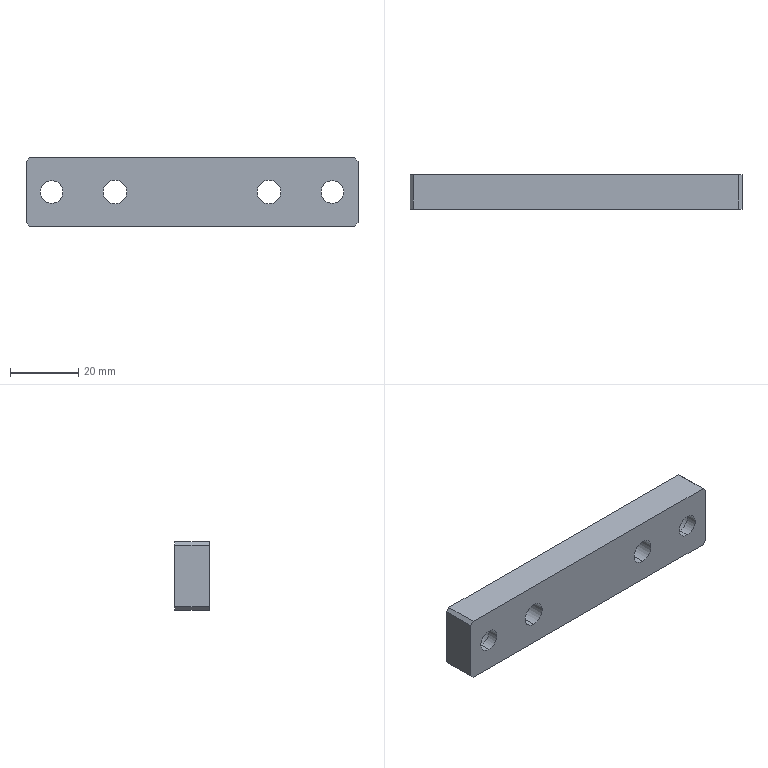Part | SolidWorks | features HoleWzd 2, Chamfer 1, Extrusion 1, ICE 1 | 1 solid | 24 faces | box 97 x 10 x 20 mm | volume 17099 mm3 | cylinder 12 | plane 12 | commonest cylinder face diameters 6.6 x4 7 x4 11 x4
STEP:
#1=CARTESIAN_POINT('',(-41.,-1.8,-5.5));
#2=VERTEX_POINT('',#1);
#3=CARTESIAN_POINT('',(-41.,-1.8,5.5));
#4=VERTEX_POINT('',#3);
#5=CARTESIAN_POINT('',(-41.,-1.8,0.));
#6=DIRECTION('',(0.,1.,0.));
#7=DIRECTION('',(0.,0.,1.));
#8=AXIS2_PLACEMENT_3D('',#5,#6,#7);
#9=CIRCLE('',#8,5.5);
#10=EDGE_CURVE('',#2,#4,#9,.T.);
#11=ORIENTED_EDGE('',*,*,#10,.F.);
#12=CARTESIAN_POINT('',(-41.,5.,-5.5));
#13=VERTEX_POINT('',#12);
#14=CARTESIAN_POINT('',(-41.,5.,-5.5));
#15=DIRECTION('',(0.,1.,0.));
#16=VECTOR('',#15,1000.);
#17=LINE('',#14,#16);
#18=EDGE_CURVE('',#2,#13,#17,.T.);
#19=ORIENTED_EDGE('',*,*,#18,.T.);
#20=CARTESIAN_POINT('',(-41.,5.,5.5));
#21=VERTEX_POINT('',#20);
#22=CARTESIAN_POINT('',(-41.,5.,0.));
#23=DIRECTION('',(0.,1.,0.));
#24=DIRECTION('',(0.,0.,1.));
#25=AXIS2_PLACEMENT_3D('',#22,#23,#24);
#26=CIRCLE('',#25,5.5);
#27=EDGE_CURVE('',#13,#21,#26,.T.);
#28=ORIENTED_EDGE('',*,*,#27,.T.);
#29=CARTESIAN_POINT('',(-41.,5.,5.5));
#30=DIRECTION('',(0.,1.,0.));
#31=VECTOR('',#30,1000.);
#32=LINE('',#29,#31);
#33=EDGE_CURVE('',#4,#21,#32,.T.);
#34=ORIENTED_EDGE('',*,*,#33,.F.);
#35=EDGE_LOOP('',(#11,#19,#28,#34));
#36=FACE_OUTER_BOUND('',#35,.T.);
#37=CARTESIAN_POINT('',(-41.,5.,0.));
#38=DIRECTION('',(0.,1.,0.));
#39=DIRECTION('',(0.,0.,1.));
#40=AXIS2_PLACEMENT_3D('',#37,#38,#39);
#41=CYLINDRICAL_SURFACE('',#40,5.5);
#42=ADVANCED_FACE('',(#36),#41,.F.);
#43=CARTESIAN_POINT('',(-41.,-5.,-3.3));
#44=VERTEX_POINT('',#43);
#45=CARTESIAN_POINT('',(-41.,-5.,3.3));
#46=VERTEX_POINT('',#45);
#47=CARTESIAN_POINT('',(-41.,-5.,0.));
#48=DIRECTION('',(0.,1.,0.));
#49=DIRECTION('',(0.,0.,1.));
#50=AXIS2_PLACEMENT_3D('',#47,#48,#49);
#51=CIRCLE('',#50,3.3);
#52=EDGE_CURVE('',#44,#46,#51,.T.);
#53=ORIENTED_EDGE('',*,*,#52,.F.);
#54=CARTESIAN_POINT('',(-41.,-1.8,-3.3));
#55=VERTEX_POINT('',#54);
#56=CARTESIAN_POINT('',(-41.,5.,-3.3));
#57=DIRECTION('',(0.,1.,0.));
#58=VECTOR('',#57,1000.);
#59=LINE('',#56,#58);
#60=EDGE_CURVE('',#44,#55,#59,.T.);
#61=ORIENTED_EDGE('',*,*,#60,.T.);
#62=CARTESIAN_POINT('',(-41.,-1.8,3.3));
#63=VERTEX_POINT('',#62);
#64=CARTESIAN_POINT('',(-41.,-1.8,0.));
#65=DIRECTION('',(0.,1.,0.));
#66=DIRECTION('',(0.,0.,1.));
#67=AXIS2_PLACEMENT_3D('',#64,#65,#66);
#68=CIRCLE('',#67,3.3);
#69=EDGE_CURVE('',#55,#63,#68,.T.);
#70=ORIENTED_EDGE('',*,*,#69,.T.);
#71=CARTESIAN_POINT('',(-41.,5.,3.3));
#72=DIRECTION('',(0.,1.,0.));
#73=VECTOR('',#72,1000.);
#74=LINE('',#71,#73);
#75=EDGE_CURVE('',#46,#63,#74,.T.);
#76=ORIENTED_EDGE('',*,*,#75,.F.);
#77=EDGE_LOOP('',(#53,#61,#70,#76));
#78=FACE_OUTER_BOUND('',#77,.T.);
#79=CARTESIAN_POINT('',(-41.,5.,0.));
#80=DIRECTION('',(0.,1.,0.));
#81=DIRECTION('',(0.,0.,1.));
#82=AXIS2_PLACEMENT_3D('',#79,#80,#81);
#83=CYLINDRICAL_SURFACE('',#82,3.3);
#84=ADVANCED_FACE('',(#78),#83,.F.);
#85=CARTESIAN_POINT('',(41.,-1.8,-5.5));
#86=VERTEX_POINT('',#85);
#87=CARTESIAN_POINT('',(41.,-1.8,5.5));
#88=VERTEX_POINT('',#87);
#89=CARTESIAN_POINT('',(41.,-1.8,0.));
#90=DIRECTION('',(0.,1.,0.));
#91=DIRECTION('',(0.,0.,1.));
#92=AXIS2_PLACEMENT_3D('',#89,#90,#91);
#93=CIRCLE('',#92,5.5);
#94=EDGE_CURVE('',#86,#88,#93,.T.);
#95=ORIENTED_EDGE('',*,*,#94,.F.);
#96=CARTESIAN_POINT('',(41.,5.,-5.5));
#97=VERTEX_POINT('',#96);
#98=CARTESIAN_POINT('',(41.,5.,-5.5));
#99=DIRECTION('',(0.,1.,0.));
#100=VECTOR('',#99,1000.);
#101=LINE('',#98,#100);
#102=EDGE_CURVE('',#86,#97,#101,.T.);
#103=ORIENTED_EDGE('',*,*,#102,.T.);
#104=CARTESIAN_POINT('',(41.,5.,5.5));
#105=VERTEX_POINT('',#104);
#106=CARTESIAN_POINT('',(41.,5.,0.));
#107=DIRECTION('',(0.,1.,0.));
#108=DIRECTION('',(0.,0.,1.));
#109=AXIS2_PLACEMENT_3D('',#106,#107,#108);
#110=CIRCLE('',#109,5.5);
#111=EDGE_CURVE('',#97,#105,#110,.T.);
#112=ORIENTED_EDGE('',*,*,#111,.T.);
#113=CARTESIAN_POINT('',(41.,5.,5.5));
#114=DIRECTION('',(0.,1.,0.));
#115=VECTOR('',#114,1000.);
#116=LINE('',#113,#115);
#117=EDGE_CURVE('',#88,#105,#116,.T.);
#118=ORIENTED_EDGE('',*,*,#117,.F.);
#119=EDGE_LOOP('',(#95,#103,#112,#118));
#120=FACE_OUTER_BOUND('',#119,.T.);
#121=CARTESIAN_POINT('',(41.,5.,0.));
#122=DIRECTION('',(0.,1.,0.));
#123=DIRECTION('',(0.,0.,1.));
#124=AXIS2_PLACEMENT_3D('',#121,#122,#123);
#125=CYLINDRICAL_SURFACE('',#124,5.5);
#126=ADVANCED_FACE('',(#120),#125,.F.);
#127=CARTESIAN_POINT('',(41.,-5.,-3.3));
#128=VERTEX_POINT('',#127);
#129=CARTESIAN_POINT('',(41.,-5.,3.3));
#130=VERTEX_POINT('',#129);
#131=CARTESIAN_POINT('',(41.,-5.,0.));
#132=DIRECTION('',(0.,1.,0.));
#133=DIRECTION('',(0.,0.,1.));
#134=AXIS2_PLACEMENT_3D('',#131,#132,#133);
#135=CIRCLE('',#134,3.3);
#136=EDGE_CURVE('',#128,#130,#135,.T.);
#137=ORIENTED_EDGE('',*,*,#136,.F.);
#138=CARTESIAN_POINT('',(41.,-1.8,-3.3));
#139=VERTEX_POINT('',#138);
#140=CARTESIAN_POINT('',(41.,5.,-3.3));
#141=DIRECTION('',(0.,1.,0.));
#142=VECTOR('',#141,1000.);
#143=LINE('',#140,#142);
#144=EDGE_CURVE('',#128,#139,#143,.T.);
#145=ORIENTED_EDGE('',*,*,#144,.T.);
#146=CARTESIAN_POINT('',(41.,-1.8,3.3));
#147=VERTEX_POINT('',#146);
#148=CARTESIAN_POINT('',(41.,-1.8,0.));
#149=DIRECTION('',(0.,1.,0.));
#150=DIRECTION('',(0.,0.,1.));
#151=AXIS2_PLACEMENT_3D('',#148,#149,#150);
#152=CIRCLE('',#151,3.3);
#153=EDGE_CURVE('',#139,#147,#152,.T.);
#154=ORIENTED_EDGE('',*,*,#153,.T.);
#155=CARTESIAN_POINT('',(41.,5.,3.3));
#156=DIRECTION('',(0.,1.,0.));
#157=VECTOR('',#156,1000.);
#158=LINE('',#155,#157);
#159=EDGE_CURVE('',#130,#147,#158,.T.);
#160=ORIENTED_EDGE('',*,*,#159,.F.);
#161=EDGE_LOOP('',(#137,#145,#154,#160));
#162=FACE_OUTER_BOUND('',#161,.T.);
#163=CARTESIAN_POINT('',(41.,5.,0.));
#164=DIRECTION('',(0.,1.,0.));
#165=DIRECTION('',(0.,0.,1.));
#166=AXIS2_PLACEMENT_3D('',#163,#164,#165);
#167=CYLINDRICAL_SURFACE('',#166,3.3);
#168=ADVANCED_FACE('',(#162),#167,.F.);
#169=CARTESIAN_POINT('',(-22.5,-5.,-3.5));
#170=VERTEX_POINT('',#169);
#171=CARTESIAN_POINT('',(-22.5,-5.,3.5));
#172=VERTEX_POINT('',#171);
#173=CARTESIAN_POINT('',(-22.5,-5.,0.));
#174=DIRECTION('',(0.,1.,0.));
#175=DIRECTION('',(0.,0.,1.));
#176=AXIS2_PLACEMENT_3D('',#173,#174,#175);
#177=CIRCLE('',#176,3.5);
#178=EDGE_CURVE('',#170,#172,#177,.T.);
#179=ORIENTED_EDGE('',*,*,#178,.F.);
#180=CARTESIAN_POINT('',(-22.5,5.,-3.5));
#181=VERTEX_POINT('',#180);
#182=CARTESIAN_POINT('',(-22.5,5.,-3.5));
#183=DIRECTION('',(0.,1.,0.));
#184=VECTOR('',#183,1000.);
#185=LINE('',#182,#184);
#186=EDGE_CURVE('',#170,#181,#185,.T.);
#187=ORIENTED_EDGE('',*,*,#186,.T.);
#188=CARTESIAN_POINT('',(-22.5,5.,3.5));
#189=VERTEX_POINT('',#188);
#190=CARTESIAN_POINT('',(-22.5,5.,0.));
#191=DIRECTION('',(0.,1.,0.));
#192=DIRECTION('',(0.,0.,1.));
#193=AXIS2_PLACEMENT_3D('',#190,#191,#192);
#194=CIRCLE('',#193,3.5);
#195=EDGE_CURVE('',#181,#189,#194,.T.);
#196=ORIENTED_EDGE('',*,*,#195,.T.);
#197=CARTESIAN_POINT('',(-22.5,5.,3.5));
#198=DIRECTION('',(0.,1.,0.));
#199=VECTOR('',#198,1000.);
#200=LINE('',#197,#199);
#201=EDGE_CURVE('',#172,#189,#200,.T.);
#202=ORIENTED_EDGE('',*,*,#201,.F.);
#203=EDGE_LOOP('',(#179,#187,#196,#202));
#204=FACE_OUTER_BOUND('',#203,.T.);
#205=CARTESIAN_POINT('',(-22.5,5.,0.));
#206=DIRECTION('',(0.,1.,0.));
#207=DIRECTION('',(0.,0.,1.));
#208=AXIS2_PLACEMENT_3D('',#205,#206,#207);
#209=CYLINDRICAL_SURFACE('',#208,3.5);
#210=ADVANCED_FACE('',(#204),#209,.F.);
#211=CARTESIAN_POINT('',(22.5,-5.,-3.5));
#212=VERTEX_POINT('',#211);
#213=CARTESIAN_POINT('',(22.5,-5.,3.5));
#214=VERTEX_POINT('',#213);
#215=CARTESIAN_POINT('',(22.5,-5.,0.));
#216=DIRECTION('',(0.,1.,0.));
#217=DIRECTION('',(0.,0.,1.));
#218=AXIS2_PLACEMENT_3D('',#215,#216,#217);
#219=CIRCLE('',#218,3.5);
#220=EDGE_CURVE('',#212,#214,#219,.T.);
#221=ORIENTED_EDGE('',*,*,#220,.F.);
#222=CARTESIAN_POINT('',(22.5,5.,-3.5));
#223=VERTEX_POINT('',#222);
#224=CARTESIAN_POINT('',(22.5,5.,-3.5));
#225=DIRECTION('',(0.,1.,0.));
#226=VECTOR('',#225,1000.);
#227=LINE('',#224,#226);
#228=EDGE_CURVE('',#212,#223,#227,.T.);
#229=ORIENTED_EDGE('',*,*,#228,.T.);
#230=CARTESIAN_POINT('',(22.5,5.,3.5));
#231=VERTEX_POINT('',#230);
#232=CARTESIAN_POINT('',(22.5,5.,0.));
#233=DIRECTION('',(0.,1.,0.));
#234=DIRECTION('',(0.,0.,1.));
#235=AXIS2_PLACEMENT_3D('',#232,#233,#234);
#236=CIRCLE('',#235,3.5);
#237=EDGE_CURVE('',#223,#231,#236,.T.);
#238=ORIENTED_EDGE('',*,*,#237,.T.);
#239=CARTESIAN_POINT('',(22.5,5.,3.5));
#240=DIRECTION('',(0.,1.,0.));
#241=VECTOR('',#240,1000.);
#242=LINE('',#239,#241);
#243=EDGE_CURVE('',#214,#231,#242,.T.);
#244=ORIENTED_EDGE('',*,*,#243,.F.);
#245=EDGE_LOOP('',(#221,#229,#238,#244));
#246=FACE_OUTER_BOUND('',#245,.T.);
#247=CARTESIAN_POINT('',(22.5,5.,0.));
#248=DIRECTION('',(0.,1.,0.));
#249=DIRECTION('',(0.,0.,1.));
#250=AXIS2_PLACEMENT_3D('',#247,#248,#249);
#251=CYLINDRICAL_SURFACE('',#250,3.5);
#252=ADVANCED_FACE('',(#246),#251,.F.);
#253=CARTESIAN_POINT('',(48.5,5.,9.));
#254=VERTEX_POINT('',#253);
#255=CARTESIAN_POINT('',(48.5,5.,-9.));
#256=VERTEX_POINT('',#255);
#257=CARTESIAN_POINT('',(48.5,5.,10.));
#258=DIRECTION('',(0.,0.,-1.));
#259=VECTOR('',#258,1000.);
#260=LINE('',#257,#259);
#261=EDGE_CURVE('',#254,#256,#260,.T.);
#262=ORIENTED_EDGE('',*,*,#261,.F.);
#263=CARTESIAN_POINT('',(48.5,-5.,9.));
#264=VERTEX_POINT('',#263);
#265=CARTESIAN_POINT('',(48.5,5.,9.));
#266=DIRECTION('',(0.,-1.,0.));
#267=VECTOR('',#266,1000.);
#268=LINE('',#265,#267);
#269=EDGE_CURVE('',#254,#264,#268,.T.);
#270=ORIENTED_EDGE('',*,*,#269,.T.);
#271=CARTESIAN_POINT('',(48.5,-5.,-9.));
#272=VERTEX_POINT('',#271);
#273=CARTESIAN_POINT('',(48.5,-5.,10.));
#274=DIRECTION('',(0.,0.,-1.));
#275=VECTOR('',#274,1000.);
#276=LINE('',#273,#275);
#277=EDGE_CURVE('',#264,#272,#276,.T.);
#278=ORIENTED_EDGE('',*,*,#277,.T.);
#279=CARTESIAN_POINT('',(48.5,5.,-9.));
#280=DIRECTION('',(0.,1.,0.));
#281=VECTOR('',#280,1000.);
#282=LINE('',#279,#281);
#283=EDGE_CURVE('',#272,#256,#282,.T.);
#284=ORIENTED_EDGE('',*,*,#283,.T.);
#285=EDGE_LOOP('',(#262,#270,#278,#284));
#286=FACE_OUTER_BOUND('',#285,.T.);
#287=CARTESIAN_POINT('',(48.5,5.,10.));
#288=DIRECTION('',(-1.,0.,0.));
#289=DIRECTION('',(0.,0.,1.));
#290=AXIS2_PLACEMENT_3D('',#287,#288,#289);
#291=PLANE('',#290);
#292=ADVANCED_FACE('',(#286),#291,.F.);
#293=CARTESIAN_POINT('',(47.5,-5.,-10.));
#294=VERTEX_POINT('',#293);
#295=CARTESIAN_POINT('',(-47.5,-5.,-10.));
#296=VERTEX_POINT('',#295);
#297=CARTESIAN_POINT('',(-48.5,-5.,-10.));
#298=DIRECTION('',(-1.,0.,0.));
#299=VECTOR('',#298,1000.);
#300=LINE('',#297,#299);
#301=EDGE_CURVE('',#294,#296,#300,.T.);
#302=ORIENTED_EDGE('',*,*,#301,.T.);
#303=CARTESIAN_POINT('',(-47.5,5.,-10.));
#304=VERTEX_POINT('',#303);
#305=CARTESIAN_POINT('',(-47.5,5.,-10.));
#306=DIRECTION('',(0.,1.,0.));
#307=VECTOR('',#306,1000.);
#308=LINE('',#305,#307);
#309=EDGE_CURVE('',#296,#304,#308,.T.);
#310=ORIENTED_EDGE('',*,*,#309,.T.);
#311=CARTESIAN_POINT('',(47.5,5.,-10.));
#312=VERTEX_POINT('',#311);
#313=CARTESIAN_POINT('',(-48.5,5.,-10.));
#314=DIRECTION('',(-1.,0.,0.));
#315=VECTOR('',#314,1000.);
#316=LINE('',#313,#315);
#317=EDGE_CURVE('',#312,#304,#316,.T.);
#318=ORIENTED_EDGE('',*,*,#317,.F.);
#319=CARTESIAN_POINT('',(47.5,5.,-10.));
#320=DIRECTION('',(0.,-1.,0.));
#321=VECTOR('',#320,1000.);
#322=LINE('',#319,#321);
#323=EDGE_CURVE('',#312,#294,#322,.T.);
#324=ORIENTED_EDGE('',*,*,#323,.T.);
#325=EDGE_LOOP('',(#302,#310,#318,#324));
#326=FACE_OUTER_BOUND('',#325,.T.);
#327=CARTESIAN_POINT('',(-48.5,5.,-10.));
#328=DIRECTION('',(0.,0.,1.));
#329=DIRECTION('',(1.,0.,0.));
#330=AXIS2_PLACEMENT_3D('',#327,#328,#329);
#331=PLANE('',#330);
#332=ADVANCED_FACE('',(#326),#331,.F.);
#333=CARTESIAN_POINT('',(-48.5,-5.,-9.));
#334=VERTEX_POINT('',#333);
#335=CARTESIAN_POINT('',(-48.5,-5.,9.));
#336=VERTEX_POINT('',#335);
#337=CARTESIAN_POINT('',(-48.5,-5.,10.));
#338=DIRECTION('',(0.,0.,1.));
#339=VECTOR('',#338,1000.);
#340=LINE('',#337,#339);
#341=EDGE_CURVE('',#334,#336,#340,.T.);
#342=ORIENTED_EDGE('',*,*,#341,.T.);
#343=CARTESIAN_POINT('',(-48.5,5.,9.));
#344=VERTEX_POINT('',#343);
#345=CARTESIAN_POINT('',(-48.5,5.,9.));
#346=DIRECTION('',(0.,1.,0.));
#347=VECTOR('',#346,1000.);
#348=LINE('',#345,#347);
#349=EDGE_CURVE('',#336,#344,#348,.T.);
#350=ORIENTED_EDGE('',*,*,#349,.T.);
#351=CARTESIAN_POINT('',(-48.5,5.,-9.));
#352=VERTEX_POINT('',#351);
#353=CARTESIAN_POINT('',(-48.5,5.,10.));
#354=DIRECTION('',(0.,0.,1.));
#355=VECTOR('',#354,1000.);
#356=LINE('',#353,#355);
#357=EDGE_CURVE('',#352,#344,#356,.T.);
#358=ORIENTED_EDGE('',*,*,#357,.F.);
#359=CARTESIAN_POINT('',(-48.5,5.,-9.));
#360=DIRECTION('',(0.,-1.,0.));
#361=VECTOR('',#360,1000.);
#362=LINE('',#359,#361);
#363=EDGE_CURVE('',#352,#334,#362,.T.);
#364=ORIENTED_EDGE('',*,*,#363,.T.);
#365=EDGE_LOOP('',(#342,#350,#358,#364));
#366=FACE_OUTER_BOUND('',#365,.T.);
#367=CARTESIAN_POINT('',(-48.5,5.,10.));
#368=DIRECTION('',(1.,0.,0.));
#369=DIRECTION('',(0.,0.,-1.));
#370=AXIS2_PLACEMENT_3D('',#367,#368,#369);
#371=PLANE('',#370);
#372=ADVANCED_FACE('',(#366),#371,.F.);
#373=CARTESIAN_POINT('',(-47.5,-5.,10.));
#374=VERTEX_POINT('',#373);
#375=CARTESIAN_POINT('',(47.5,-5.,10.));
#376=VERTEX_POINT('',#375);
#377=CARTESIAN_POINT('',(-48.5,-5.,10.));
#378=DIRECTION('',(1.,0.,0.));
#379=VECTOR('',#378,1000.);
#380=LINE('',#377,#379);
#381=EDGE_CURVE('',#374,#376,#380,.T.);
#382=ORIENTED_EDGE('',*,*,#381,.T.);
#383=CARTESIAN_POINT('',(47.5,5.,10.));
#384=VERTEX_POINT('',#383);
#385=CARTESIAN_POINT('',(47.5,5.,10.));
#386=DIRECTION('',(0.,1.,0.));
#387=VECTOR('',#386,1000.);
#388=LINE('',#385,#387);
#389=EDGE_CURVE('',#376,#384,#388,.T.);
#390=ORIENTED_EDGE('',*,*,#389,.T.);
#391=CARTESIAN_POINT('',(-47.5,5.,10.));
#392=VERTEX_POINT('',#391);
#393=CARTESIAN_POINT('',(-48.5,5.,10.));
#394=DIRECTION('',(1.,0.,0.));
#395=VECTOR('',#394,1000.);
#396=LINE('',#393,#395);
#397=EDGE_CURVE('',#392,#384,#396,.T.);
#398=ORIENTED_EDGE('',*,*,#397,.F.);
#399=CARTESIAN_POINT('',(-47.5,5.,10.));
#400=DIRECTION('',(0.,-1.,0.));
#401=VECTOR('',#400,1000.);
#402=LINE('',#399,#401);
#403=EDGE_CURVE('',#392,#374,#402,.T.);
#404=ORIENTED_EDGE('',*,*,#403,.T.);
#405=EDGE_LOOP('',(#382,#390,#398,#404));
#406=FACE_OUTER_BOUND('',#405,.T.);
#407=CARTESIAN_POINT('',(-48.5,5.,10.));
#408=DIRECTION('',(0.,0.,-1.));
#409=DIRECTION('',(-1.,0.,0.));
#410=AXIS2_PLACEMENT_3D('',#407,#408,#409);
#411=PLANE('',#410);
#412=ADVANCED_FACE('',(#406),#411,.F.);
#413=CARTESIAN_POINT('',(-41.,5.,0.));
#414=DIRECTION('',(0.,1.,0.));
#415=DIRECTION('',(0.,0.,1.));
#416=AXIS2_PLACEMENT_3D('',#413,#414,#415);
#417=CIRCLE('',#416,5.5);
#418=EDGE_CURVE('',#21,#13,#417,.T.);
#419=ORIENTED_EDGE('',*,*,#418,.F.);
#420=ORIENTED_EDGE('',*,*,#27,.F.);
#421=EDGE_LOOP('',(#419,#420));
#422=FACE_BOUND('',#421,.T.);
#423=CARTESIAN_POINT('',(41.,5.,0.));
#424=DIRECTION('',(0.,1.,0.));
#425=DIRECTION('',(0.,0.,1.));
#426=AXIS2_PLACEMENT_3D('',#423,#424,#425);
#427=CIRCLE('',#426,5.5);
#428=EDGE_CURVE('',#105,#97,#427,.T.);
#429=ORIENTED_EDGE('',*,*,#428,.F.);
#430=ORIENTED_EDGE('',*,*,#111,.F.);
#431=EDGE_LOOP('',(#429,#430));
#432=FACE_BOUND('',#431,.T.);
#433=CARTESIAN_POINT('',(-22.5,5.,0.));
#434=DIRECTION('',(0.,1.,0.));
#435=DIRECTION('',(0.,0.,1.));
#436=AXIS2_PLACEMENT_3D('',#433,#434,#435);
#437=CIRCLE('',#436,3.5);
#438=EDGE_CURVE('',#189,#181,#437,.T.);
#439=ORIENTED_EDGE('',*,*,#438,.F.);
#440=ORIENTED_EDGE('',*,*,#195,.F.);
#441=EDGE_LOOP('',(#439,#440));
#442=FACE_BOUND('',#441,.T.);
#443=CARTESIAN_POINT('',(22.5,5.,0.));
#444=DIRECTION('',(0.,1.,0.));
#445=DIRECTION('',(0.,0.,1.));
#446=AXIS2_PLACEMENT_3D('',#443,#444,#445);
#447=CIRCLE('',#446,3.5);
#448=EDGE_CURVE('',#231,#223,#447,.T.);
#449=ORIENTED_EDGE('',*,*,#448,.F.);
#450=ORIENTED_EDGE('',*,*,#237,.F.);
#451=EDGE_LOOP('',(#449,#450));
#452=FACE_BOUND('',#451,.T.);
#453=ORIENTED_EDGE('',*,*,#397,.T.);
#454=CARTESIAN_POINT('',(48.5,5.,9.));
#455=DIRECTION('',(0.7071,0.,-0.7071));
#456=VECTOR('',#455,1000.);
#457=LINE('',#454,#456);
#458=EDGE_CURVE('',#384,#254,#457,.T.);
#459=ORIENTED_EDGE('',*,*,#458,.T.);
#460=ORIENTED_EDGE('',*,*,#261,.T.);
#461=CARTESIAN_POINT('',(47.5,5.,-10.));
#462=DIRECTION('',(-0.7071,0.,-0.7071));
#463=VECTOR('',#462,1000.);
#464=LINE('',#461,#463);
#465=EDGE_CURVE('',#256,#312,#464,.T.);
#466=ORIENTED_EDGE('',*,*,#465,.T.);
#467=ORIENTED_EDGE('',*,*,#317,.T.);
#468=CARTESIAN_POINT('',(-48.5,5.,-9.));
#469=DIRECTION('',(-0.7071,0.,0.7071));
#470=VECTOR('',#469,1000.);
#471=LINE('',#468,#470);
#472=EDGE_CURVE('',#304,#352,#471,.T.);
#473=ORIENTED_EDGE('',*,*,#472,.T.);
#474=ORIENTED_EDGE('',*,*,#357,.T.);
#475=CARTESIAN_POINT('',(-47.5,5.,10.));
#476=DIRECTION('',(0.7071,0.,0.7071));
#477=VECTOR('',#476,1000.);
#478=LINE('',#475,#477);
#479=EDGE_CURVE('',#344,#392,#478,.T.);
#480=ORIENTED_EDGE('',*,*,#479,.T.);
#481=EDGE_LOOP('',(#453,#459,#460,#466,#467,#473,#474,#480));
#482=FACE_OUTER_BOUND('',#481,.T.);
#483=CARTESIAN_POINT('',(0.,5.,0.));
#484=DIRECTION('',(0.,-1.,0.));
#485=DIRECTION('',(0.,0.,-1.));
#486=AXIS2_PLACEMENT_3D('',#483,#484,#485);
#487=PLANE('',#486);
#488=ADVANCED_FACE('',(#422,#432,#442,#452,#482),#487,.F.);
#489=CARTESIAN_POINT('',(-41.,-5.,0.));
#490=DIRECTION('',(0.,1.,0.));
#491=DIRECTION('',(0.,0.,1.));
#492=AXIS2_PLACEMENT_3D('',#489,#490,#491);
#493=CIRCLE('',#492,3.3);
#494=EDGE_CURVE('',#46,#44,#493,.T.);
#495=ORIENTED_EDGE('',*,*,#494,.T.);
#496=ORIENTED_EDGE('',*,*,#52,.T.);
#497=EDGE_LOOP('',(#495,#496));
#498=FACE_BOUND('',#497,.T.);
#499=CARTESIAN_POINT('',(41.,-5.,0.));
#500=DIRECTION('',(0.,1.,0.));
#501=DIRECTION('',(0.,0.,1.));
#502=AXIS2_PLACEMENT_3D('',#499,#500,#501);
#503=CIRCLE('',#502,3.3);
#504=EDGE_CURVE('',#130,#128,#503,.T.);
#505=ORIENTED_EDGE('',*,*,#504,.T.);
#506=ORIENTED_EDGE('',*,*,#136,.T.);
#507=EDGE_LOOP('',(#505,#506));
#508=FACE_BOUND('',#507,.T.);
#509=CARTESIAN_POINT('',(-22.5,-5.,0.));
#510=DIRECTION('',(0.,1.,0.));
#511=DIRECTION('',(0.,0.,1.));
#512=AXIS2_PLACEMENT_3D('',#509,#510,#511);
#513=CIRCLE('',#512,3.5);
#514=EDGE_CURVE('',#172,#170,#513,.T.);
#515=ORIENTED_EDGE('',*,*,#514,.T.);
#516=ORIENTED_EDGE('',*,*,#178,.T.);
#517=EDGE_LOOP('',(#515,#516));
#518=FACE_BOUND('',#517,.T.);
#519=CARTESIAN_POINT('',(22.5,-5.,0.));
#520=DIRECTION('',(0.,1.,0.));
#521=DIRECTION('',(0.,0.,1.));
#522=AXIS2_PLACEMENT_3D('',#519,#520,#521);
#523=CIRCLE('',#522,3.5);
#524=EDGE_CURVE('',#214,#212,#523,.T.);
#525=ORIENTED_EDGE('',*,*,#524,.T.);
#526=ORIENTED_EDGE('',*,*,#220,.T.);
#527=EDGE_LOOP('',(#525,#526));
#528=FACE_BOUND('',#527,.T.);
#529=ORIENTED_EDGE('',*,*,#277,.F.);
#530=CARTESIAN_POINT('',(28.75,-5.,28.75));
#531=DIRECTION('',(-0.7071,0.,0.7071));
#532=VECTOR('',#531,1000.);
#533=LINE('',#530,#532);
#534=EDGE_CURVE('',#264,#376,#533,.T.);
#535=ORIENTED_EDGE('',*,*,#534,.T.);
#536=ORIENTED_EDGE('',*,*,#381,.F.);
#537=CARTESIAN_POINT('',(-28.75,-5.,28.75));
#538=DIRECTION('',(-0.7071,0.,-0.7071));
#539=VECTOR('',#538,1000.);
#540=LINE('',#537,#539);
#541=EDGE_CURVE('',#374,#336,#540,.T.);
#542=ORIENTED_EDGE('',*,*,#541,.T.);
#543=ORIENTED_EDGE('',*,*,#341,.F.);
#544=CARTESIAN_POINT('',(-28.75,-5.,-28.75));
#545=DIRECTION('',(0.7071,0.,-0.7071));
#546=VECTOR('',#545,1000.);
#547=LINE('',#544,#546);
#548=EDGE_CURVE('',#334,#296,#547,.T.);
#549=ORIENTED_EDGE('',*,*,#548,.T.);
#550=ORIENTED_EDGE('',*,*,#301,.F.);
#551=CARTESIAN_POINT('',(28.75,-5.,-28.75));
#552=DIRECTION('',(0.7071,0.,0.7071));
#553=VECTOR('',#552,1000.);
#554=LINE('',#551,#553);
#555=EDGE_CURVE('',#294,#272,#554,.T.);
#556=ORIENTED_EDGE('',*,*,#555,.T.);
#557=EDGE_LOOP('',(#529,#535,#536,#542,#543,#549,#550,#556));
#558=FACE_OUTER_BOUND('',#557,.T.);
#559=CARTESIAN_POINT('',(0.,-5.,0.));
#560=DIRECTION('',(0.,-1.,0.));
#561=DIRECTION('',(0.,0.,-1.));
#562=AXIS2_PLACEMENT_3D('',#559,#560,#561);
#563=PLANE('',#562);
#564=ADVANCED_FACE('',(#498,#508,#518,#528,#558),#563,.T.);
#565=ORIENTED_EDGE('',*,*,#228,.F.);
#566=ORIENTED_EDGE('',*,*,#524,.F.);
#567=ORIENTED_EDGE('',*,*,#243,.T.);
#568=ORIENTED_EDGE('',*,*,#448,.T.);
#569=EDGE_LOOP('',(#565,#566,#567,#568));
#570=FACE_OUTER_BOUND('',#569,.T.);
#571=CARTESIAN_POINT('',(22.5,5.,0.));
#572=DIRECTION('',(0.,1.,0.));
#573=DIRECTION('',(0.,0.,1.));
#574=AXIS2_PLACEMENT_3D('',#571,#572,#573);
#575=CYLINDRICAL_SURFACE('',#574,3.5);
#576=ADVANCED_FACE('',(#570),#575,.F.);
#577=ORIENTED_EDGE('',*,*,#186,.F.);
#578=ORIENTED_EDGE('',*,*,#514,.F.);
#579=ORIENTED_EDGE('',*,*,#201,.T.);
#580=ORIENTED_EDGE('',*,*,#438,.T.);
#581=EDGE_LOOP('',(#577,#578,#579,#580));
#582=FACE_OUTER_BOUND('',#581,.T.);
#583=CARTESIAN_POINT('',(-22.5,5.,0.));
#584=DIRECTION('',(0.,1.,0.));
#585=DIRECTION('',(0.,0.,1.));
#586=AXIS2_PLACEMENT_3D('',#583,#584,#585);
#587=CYLINDRICAL_SURFACE('',#586,3.5);
#588=ADVANCED_FACE('',(#582),#587,.F.);
#589=ORIENTED_EDGE('',*,*,#144,.F.);
#590=ORIENTED_EDGE('',*,*,#504,.F.);
#591=ORIENTED_EDGE('',*,*,#159,.T.);
#592=CARTESIAN_POINT('',(41.,-1.8,0.));
#593=DIRECTION('',(0.,1.,0.));
#594=DIRECTION('',(0.,0.,1.));
#595=AXIS2_PLACEMENT_3D('',#592,#593,#594);
#596=CIRCLE('',#595,3.3);
#597=EDGE_CURVE('',#147,#139,#596,.T.);
#598=ORIENTED_EDGE('',*,*,#597,.T.);
#599=EDGE_LOOP('',(#589,#590,#591,#598));
#600=FACE_OUTER_BOUND('',#599,.T.);
#601=CARTESIAN_POINT('',(41.,5.,0.));
#602=DIRECTION('',(0.,1.,0.));
#603=DIRECTION('',(0.,0.,1.));
#604=AXIS2_PLACEMENT_3D('',#601,#602,#603);
#605=CYLINDRICAL_SURFACE('',#604,3.3);
#606=ADVANCED_FACE('',(#600),#605,.F.);
#607=ORIENTED_EDGE('',*,*,#597,.F.);
#608=ORIENTED_EDGE('',*,*,#153,.F.);
#609=EDGE_LOOP('',(#607,#608));
#610=FACE_BOUND('',#609,.T.);
#611=CARTESIAN_POINT('',(41.,-1.8,0.));
#612=DIRECTION('',(0.,1.,0.));
#613=DIRECTION('',(0.,0.,1.));
#614=AXIS2_PLACEMENT_3D('',#611,#612,#613);
#615=CIRCLE('',#614,5.5);
#616=EDGE_CURVE('',#88,#86,#615,.T.);
#617=ORIENTED_EDGE('',*,*,#616,.T.);
#618=ORIENTED_EDGE('',*,*,#94,.T.);
#619=EDGE_LOOP('',(#617,#618));
#620=FACE_OUTER_BOUND('',#619,.T.);
#621=CARTESIAN_POINT('',(44.3,-1.8,0.));
#622=DIRECTION('',(0.,-1.,0.));
#623=DIRECTION('',(0.,0.,-1.));
#624=AXIS2_PLACEMENT_3D('',#621,#622,#623);
#625=PLANE('',#624);
#626=ADVANCED_FACE('',(#610,#620),#625,.F.);
#627=ORIENTED_EDGE('',*,*,#102,.F.);
#628=ORIENTED_EDGE('',*,*,#616,.F.);
#629=ORIENTED_EDGE('',*,*,#117,.T.);
#630=ORIENTED_EDGE('',*,*,#428,.T.);
#631=EDGE_LOOP('',(#627,#628,#629,#630));
#632=FACE_OUTER_BOUND('',#631,.T.);
#633=CARTESIAN_POINT('',(41.,5.,0.));
#634=DIRECTION('',(0.,1.,0.));
#635=DIRECTION('',(0.,0.,1.));
#636=AXIS2_PLACEMENT_3D('',#633,#634,#635);
#637=CYLINDRICAL_SURFACE('',#636,5.5);
#638=ADVANCED_FACE('',(#632),#637,.F.);
#639=ORIENTED_EDGE('',*,*,#60,.F.);
#640=ORIENTED_EDGE('',*,*,#494,.F.);
#641=ORIENTED_EDGE('',*,*,#75,.T.);
#642=CARTESIAN_POINT('',(-41.,-1.8,0.));
#643=DIRECTION('',(0.,1.,0.));
#644=DIRECTION('',(0.,0.,1.));
#645=AXIS2_PLACEMENT_3D('',#642,#643,#644);
#646=CIRCLE('',#645,3.3);
#647=EDGE_CURVE('',#63,#55,#646,.T.);
#648=ORIENTED_EDGE('',*,*,#647,.T.);
#649=EDGE_LOOP('',(#639,#640,#641,#648));
#650=FACE_OUTER_BOUND('',#649,.T.);
#651=CARTESIAN_POINT('',(-41.,5.,0.));
#652=DIRECTION('',(0.,1.,0.));
#653=DIRECTION('',(0.,0.,1.));
#654=AXIS2_PLACEMENT_3D('',#651,#652,#653);
#655=CYLINDRICAL_SURFACE('',#654,3.3);
#656=ADVANCED_FACE('',(#650),#655,.F.);
#657=ORIENTED_EDGE('',*,*,#647,.F.);
#658=ORIENTED_EDGE('',*,*,#69,.F.);
#659=EDGE_LOOP('',(#657,#658));
#660=FACE_BOUND('',#659,.T.);
#661=CARTESIAN_POINT('',(-41.,-1.8,0.));
#662=DIRECTION('',(0.,1.,0.));
#663=DIRECTION('',(0.,0.,1.));
#664=AXIS2_PLACEMENT_3D('',#661,#662,#663);
#665=CIRCLE('',#664,5.5);
#666=EDGE_CURVE('',#4,#2,#665,.T.);
#667=ORIENTED_EDGE('',*,*,#666,.T.);
#668=ORIENTED_EDGE('',*,*,#10,.T.);
#669=EDGE_LOOP('',(#667,#668));
#670=FACE_OUTER_BOUND('',#669,.T.);
#671=CARTESIAN_POINT('',(-37.7,-1.8,0.));
#672=DIRECTION('',(0.,-1.,0.));
#673=DIRECTION('',(0.,0.,-1.));
#674=AXIS2_PLACEMENT_3D('',#671,#672,#673);
#675=PLANE('',#674);
#676=ADVANCED_FACE('',(#660,#670),#675,.F.);
#677=ORIENTED_EDGE('',*,*,#18,.F.);
#678=ORIENTED_EDGE('',*,*,#666,.F.);
#679=ORIENTED_EDGE('',*,*,#33,.T.);
#680=ORIENTED_EDGE('',*,*,#418,.T.);
#681=EDGE_LOOP('',(#677,#678,#679,#680));
#682=FACE_OUTER_BOUND('',#681,.T.);
#683=CARTESIAN_POINT('',(-41.,5.,0.));
#684=DIRECTION('',(0.,1.,0.));
#685=DIRECTION('',(0.,0.,1.));
#686=AXIS2_PLACEMENT_3D('',#683,#684,#685);
#687=CYLINDRICAL_SURFACE('',#686,5.5);
#688=ADVANCED_FACE('',(#682),#687,.F.);
#689=ORIENTED_EDGE('',*,*,#458,.F.);
#690=ORIENTED_EDGE('',*,*,#389,.F.);
#691=ORIENTED_EDGE('',*,*,#534,.F.);
#692=ORIENTED_EDGE('',*,*,#269,.F.);
#693=EDGE_LOOP('',(#689,#690,#691,#692));
#694=FACE_OUTER_BOUND('',#693,.T.);
#695=CARTESIAN_POINT('',(48.5,5.,9.));
#696=DIRECTION('',(-0.7071,0.,-0.7071));
#697=DIRECTION('',(0.,-1.,0.));
#698=AXIS2_PLACEMENT_3D('',#695,#696,#697);
#699=PLANE('',#698);
#700=ADVANCED_FACE('',(#694),#699,.F.);
#701=ORIENTED_EDGE('',*,*,#479,.F.);
#702=ORIENTED_EDGE('',*,*,#349,.F.);
#703=ORIENTED_EDGE('',*,*,#541,.F.);
#704=ORIENTED_EDGE('',*,*,#403,.F.);
#705=EDGE_LOOP('',(#701,#702,#703,#704));
#706=FACE_OUTER_BOUND('',#705,.T.);
#707=CARTESIAN_POINT('',(-47.5,5.,10.));
#708=DIRECTION('',(0.7071,0.,-0.7071));
#709=DIRECTION('',(0.,-1.,0.));
#710=AXIS2_PLACEMENT_3D('',#707,#708,#709);
#711=PLANE('',#710);
#712=ADVANCED_FACE('',(#706),#711,.F.);
#713=ORIENTED_EDGE('',*,*,#472,.F.);
#714=ORIENTED_EDGE('',*,*,#309,.F.);
#715=ORIENTED_EDGE('',*,*,#548,.F.);
#716=ORIENTED_EDGE('',*,*,#363,.F.);
#717=EDGE_LOOP('',(#713,#714,#715,#716));
#718=FACE_OUTER_BOUND('',#717,.T.);
#719=CARTESIAN_POINT('',(-48.5,5.,-9.));
#720=DIRECTION('',(0.7071,0.,0.7071));
#721=DIRECTION('',(0.,-1.,0.));
#722=AXIS2_PLACEMENT_3D('',#719,#720,#721);
#723=PLANE('',#722);
#724=ADVANCED_FACE('',(#718),#723,.F.);
#725=ORIENTED_EDGE('',*,*,#465,.F.);
#726=ORIENTED_EDGE('',*,*,#283,.F.);
#727=ORIENTED_EDGE('',*,*,#555,.F.);
#728=ORIENTED_EDGE('',*,*,#323,.F.);
#729=EDGE_LOOP('',(#725,#726,#727,#728));
#730=FACE_OUTER_BOUND('',#729,.T.);
#731=CARTESIAN_POINT('',(47.5,5.,-10.));
#732=DIRECTION('',(-0.7071,0.,0.7071));
#733=DIRECTION('',(0.,-1.,0.));
#734=AXIS2_PLACEMENT_3D('',#731,#732,#733);
#735=PLANE('',#734);
#736=ADVANCED_FACE('',(#730),#735,.F.);
#737=CLOSED_SHELL('',(#42,#84,#126,#168,#210,#252,#292,#332,#372,#412,#488,#564,#576,#588,#606,#626,#638,#656,#676,#688,#700,#712,#724,#736));
#738=MANIFOLD_SOLID_BREP('',#737);
#739=CARTESIAN_POINT('',(0.,0.,0.));
#740=DIRECTION('',(0.,0.,1.));
#741=DIRECTION('',(1.,0.,0.));
#742=AXIS2_PLACEMENT_3D('',#739,#740,#741);
#743=(LENGTH_UNIT()NAMED_UNIT(*)SI_UNIT(.MILLI.,.METRE.));
#744=UNCERTAINTY_MEASURE_WITH_UNIT(LENGTH_MEASURE(0.00001),#743,'','');
#745=(NAMED_UNIT(*)PLANE_ANGLE_UNIT()SI_UNIT($,.RADIAN.));
#746=(NAMED_UNIT(*)SI_UNIT($,.STERADIAN.)SOLID_ANGLE_UNIT());
#747=(GEOMETRIC_REPRESENTATION_CONTEXT(3)GLOBAL_UNCERTAINTY_ASSIGNED_CONTEXT((#744))GLOBAL_UNIT_ASSIGNED_CONTEXT((#743,#745,#746))REPRESENTATION_CONTEXT('',''));
#748=ADVANCED_BREP_SHAPE_REPRESENTATION('',(#738,#742),#747);